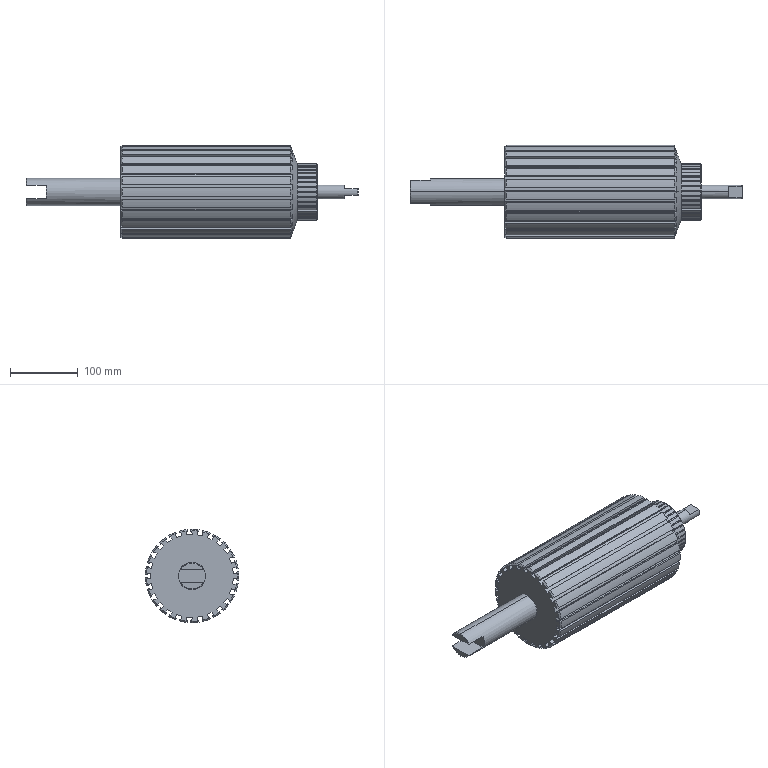Part | SolidWorks | 1 solid | 464 faces | box 490 x 137.955 x 138 mm | volume 3818604 mm3 | plane 292 | cylinder 101 | cone 71 | commonest cylinder face diameters 83.05 x36 79 x35 138 x26 20 x2 40 x2